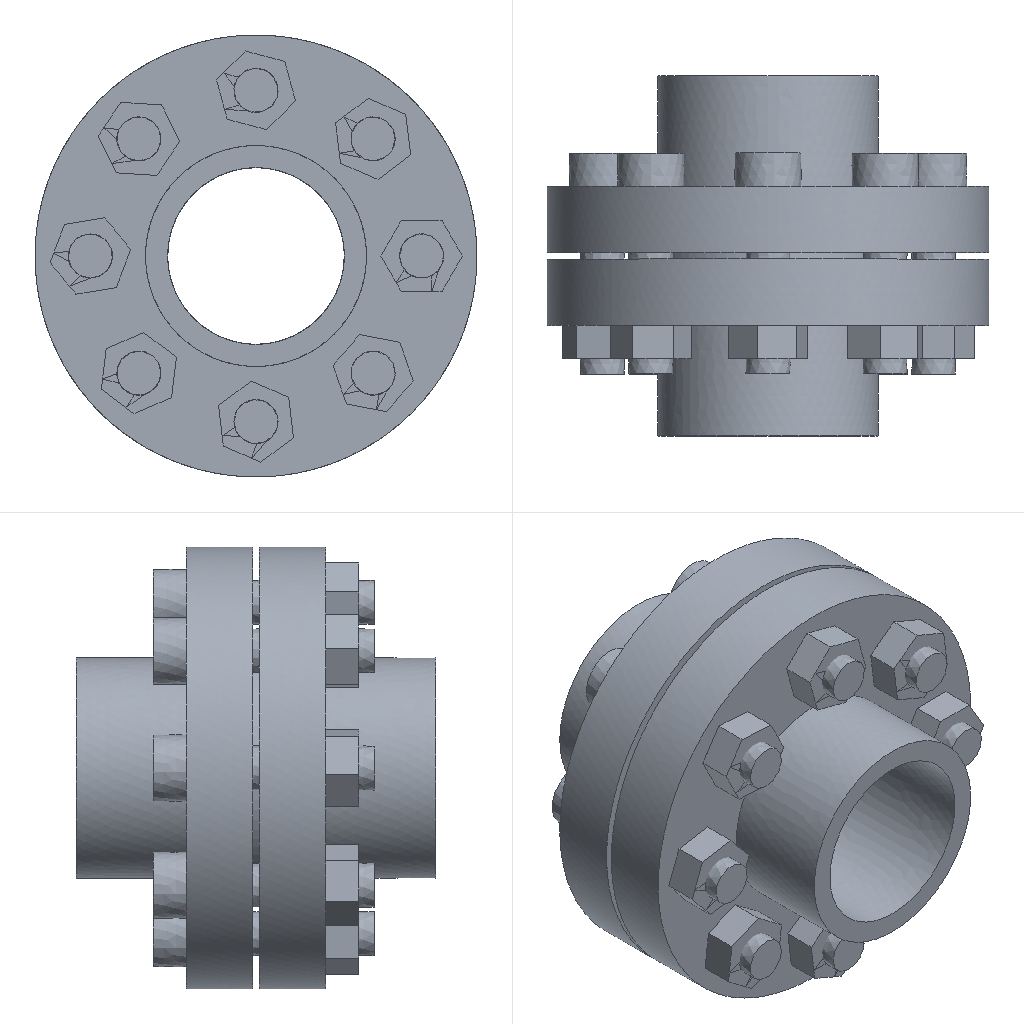Simulation study | ansys workbench
Set-up summary:
category,name,step,type,value,unit,region
solver,ansys_workbench
units,mm-N-s-tonne (MPa),,stated,"/units,MPA"
analysis,LS1,,static
load_step,LS1,LS1,static,nsubst=1; time=1
load_step,LS2,LS2,static,nsubst=1; time=2
mesh,nodes,,,148015
mesh,elements,,,97860
element_type,SOLID187,,,87205
element_type,SURF154,,,4076
element_type,TARGE170,,,2874
element_type,CONTA174,,,2874
element_type,SOLID186,,,831
material,Structural Steel,,E,200000,tonne s^-2 mm^-1
material,Structural Steel,,nu,0.3
material,Structural Steel,,density,7.85e-09,tonne mm^-3
material,Structural Steel,,conductivity,60.5,tonne mm s^-3 C^-1
material,Structural Steel,,specific_heat,4.34e+08,mm^2 s^-2 C^-1
material,Structural Steel,,cte,1.2e-05,C^-1
material,Structural Steel,,permeability,10000
material,Structural Steel,,resistivity,0.00017,ohm mm
material,Y?,,E,43,tonne s^-2 mm^-1
material,Y?,,nu,0.4995
material,Y?,,density,1.2e-09,tonne mm^-3
load,Define Pressure Using Surface Effect Elements,LS1,pressure,0.6,,SURF154 #56
load,Define Force Using Surface Effect Elements,LS1,surface-effect pres face 2,-11.318,,SURF154 #57
load,Define Force Using Surface Effect Elements,LS1,surface-effect pres face 2,-19.806,,SURF154 #58
load,Define Force Using Surface Effect Elements,LS1,surface-effect pres face 2,-19.806,,SURF154 #59
load,Define Force Using Surface Effect Elements,LS1,surface-effect pres face 2,-19.806,,SURF154 #60
load,Define Force Using Surface Effect Elements,LS1,surface-effect pres face 2,-28.295,,SURF154 #61
load,Define Force Using Surface Effect Elements,LS1,surface-effect pres face 2,-19.806,,SURF154 #62
load,Define Force Using Surface Effect Elements,LS1,surface-effect pres face 2,-19.806,,SURF154 #63
load,Define Force Using Surface Effect Elements,LS1,surface-effect pres face 2,-19.806,,SURF154 #64
bc,Fixed Supports,model,fixed,[dofs=ALL],,_FIXEDSU
contact,Contact Region,,bonded (always),element=CONTA174
contact,Contact Region 2,,bonded (always),element=CONTA174
contact,Contact Region 3,,bonded (always),element=CONTA174
contact,Contact Region 4,,bonded (always),element=CONTA174
contact,Contact Region 5,,bonded (always),element=CONTA174
contact,Contact Region 6,,bonded (always),element=CONTA174
contact,Contact Region 7,,bonded (always),element=CONTA174
contact,Contact Region 8,,bonded (always),element=CONTA174
contact,Contact Region,,bonded (always),element=CONTA174
contact,Contact Region 2,,bonded (always),element=CONTA174
contact,Contact Region 3,,bonded (always),element=CONTA174
contact,Contact Region 4,,bonded (always),element=CONTA174
contact,Contact Region 5,,bonded (always),element=CONTA174
contact,Contact Region 6,,bonded (always),element=CONTA174
contact,Contact Region 7,,bonded (always),element=CONTA174
contact,Contact Region 8,,bonded (always),element=CONTA174
contact,Frictional - falan\____-____2 ? dianpian\____-____1,,standard (frictionless/frictional),friction=0.15; element=CONTA174
contact,Frictional - falan\____-____2 ? dianpian\____-____1,,standard (frictionless/frictional),friction=0.15; element=CONTA174
named_set,_FIXEDSU,,node,3130
Ansys APDL input file, long lists of numbers shortened:
/batch
/config,noeldb,1     ! force off writing results to database
*get,_wallstrt,active,,time,wall
! ANSYS input file written by Workbench version 2021 R1
! File used for geometry attach:
/title,________--____ (C5)
*DIM,_wb_ProjectScratch_dir,string,248
_wb_ProjectScratch_dir(1) = ''
*DIM,_wb_SolverFiles_dir,string,248
_wb_SolverFiles_dir(1) = ''
*DIM,_wb_userfiles_dir,string,248
_wb_userfiles_dir(1) = ''
/com,--- Data in consistent NMM units. See Solving Units in the help system for more information.
/units,MPA
/nopr
/wb,file,start              !  signify a WB generated input file
/prep7
! Turn off shape checking because checks already performed inside WB mesher.
! See help system for more information.
SHPP,OFF,,NOWARN
/nolist
etcon,set             ! allow ANSYS to choose best KEYOP's for 180x elements, resets any applicable keyopt to MAPDL defaults
/com,*********** Nodes for the whole assembly ***********
nblock,3,,162816
(1i9,3e20.9e3)
        1     6.900000000E+01     3.000000000E+01    -8.000000000E+00
! (148014 more lines like these left out)
-1
/wb,elem,start            !  set before creation of elements
/com,*********** Elements for Body 1 "falan\____-____2" ***********
et,1,187
eblock,19,solid,,36424
(19i9)
        1        1        1        1        0        0        0        0       10        0    14541    31996    32136    35193    35172    70338    71087    70341    70340
! (72847 more lines like these left out)
-1
/com,*********** Elements for Body 2 "falan\____-____2" ***********
et,2,187
eblock,19,solid,,36424
(19i9)
        2        2        2        2        0        0        0        0       10        0    50965    90268    90408    93465    93444   128610   129359   128613   128612
! (72847 more lines like these left out)
-1
/com,*********** Elements for Body 3 "M20-LD\____-____2" ***********
et,3,187
eblock,19,solid,,1785
(19i9)
        3        3        3        3        0        0        0        0       10        0     3549     6406     6596     6715     6599     7874     8912     7876     7875
! (3569 more lines like these left out)
-1
/com,*********** Elements for Body 4 "M20-LD\____-____2" ***********
et,4,187
eblock,19,solid,,1782
(19i9)
        4        4        4        4        0        0        0        0       10        0    10977    20599    20793    20907    20796    22051    23108    22053    22052
! (3563 more lines like these left out)
-1
/com,*********** Elements for Body 5 "M20-LD\____-____2" ***********
et,5,187
eblock,19,solid,,1769
(19i9)
        5        5        5        5        0        0        0        0       10        0     1780     3524     3528     3611     3595     5949     5982     5958     5956
! (3537 more lines like these left out)
-1
! (14 more sections like these left out)
/wb,elem,end               !  done creating elements
/com,*********** Send User Defined Coordinate System(s) ***********
csys,0
toffst,273.15,  ! Temperature offset from absolute zero
/com,*********** Set Reference Temperature ***********
tref,22.
/wb,mat,start              !  starting to send materials
/com,*********** Send Materials ***********
Temperature = 'TEMP' ! Temperature
MP,DENS,1,7.85e-09,	! tonne mm^-3
MP,ALPX,1,1.2e-05,	! C^-1
MP,C,1,434000000,	! mm^2 s^-2 C^-1
MP,KXX,1,60.5,	! tonne mm s^-3 C^-1
MP,RSVX,1,0.00017,	! ohm mm
MP,EX,1,200000,	! tonne s^-2 mm^-1
MP,NUXY,1,0.3,
MP,MURX,1,10000,
Temperature = 'TEMP' ! Temperature
MP,DENS,2,7.85e-09,	! tonne mm^-3
MP,ALPX,2,1.2e-05,	! C^-1
MP,C,2,434000000,	! mm^2 s^-2 C^-1
MP,KXX,2,60.5,	! tonne mm s^-3 C^-1
MP,RSVX,2,0.00017,	! ohm mm
MP,EX,2,200000,	! tonne s^-2 mm^-1
MP,NUXY,2,0.3,
MP,MURX,2,10000,
Temperature = 'TEMP' ! Temperature
MP,DENS,3,7.85e-09,	! tonne mm^-3
MP,ALPX,3,1.2e-05,	! C^-1
MP,C,3,434000000,	! mm^2 s^-2 C^-1
MP,KXX,3,60.5,	! tonne mm s^-3 C^-1
MP,RSVX,3,0.00017,	! ohm mm
MP,EX,3,200000,	! tonne s^-2 mm^-1
MP,NUXY,3,0.3,
MP,MURX,3,10000,
Temperature = 'TEMP' ! Temperature
MP,DENS,4,7.85e-09,	! tonne mm^-3
MP,ALPX,4,1.2e-05,	! C^-1
MP,C,4,434000000,	! mm^2 s^-2 C^-1
MP,KXX,4,60.5,	! tonne mm s^-3 C^-1
MP,RSVX,4,0.00017,	! ohm mm
MP,EX,4,200000,	! tonne s^-2 mm^-1
MP,NUXY,4,0.3,
MP,MURX,4,10000,
Temperature = 'TEMP' ! Temperature
MP,DENS,5,7.85e-09,	! tonne mm^-3
MP,ALPX,5,1.2e-05,	! C^-1
MP,C,5,434000000,	! mm^2 s^-2 C^-1
MP,KXX,5,60.5,	! tonne mm s^-3 C^-1
MP,RSVX,5,0.00017,	! ohm mm
MP,EX,5,200000,	! tonne s^-2 mm^-1
MP,NUXY,5,0.3,
MP,MURX,5,10000,
Temperature = 'TEMP' ! Temperature
MP,DENS,6,7.85e-09,	! tonne mm^-3
MP,ALPX,6,1.2e-05,	! C^-1
MP,C,6,434000000,	! mm^2 s^-2 C^-1
MP,KXX,6,60.5,	! tonne mm s^-3 C^-1
MP,RSVX,6,0.00017,	! ohm mm
MP,EX,6,200000,	! tonne s^-2 mm^-1
MP,NUXY,6,0.3,
MP,MURX,6,10000,
Temperature = 'TEMP' ! Temperature
MP,DENS,7,7.85e-09,	! tonne mm^-3
MP,ALPX,7,1.2e-05,	! C^-1
MP,C,7,434000000,	! mm^2 s^-2 C^-1
MP,KXX,7,60.5,	! tonne mm s^-3 C^-1
MP,RSVX,7,0.00017,	! ohm mm
MP,EX,7,200000,	! tonne s^-2 mm^-1
MP,NUXY,7,0.3,
MP,MURX,7,10000,
Temperature = 'TEMP' ! Temperature
MP,DENS,8,7.85e-09,	! tonne mm^-3
MP,ALPX,8,1.2e-05,	! C^-1
MP,C,8,434000000,	! mm^2 s^-2 C^-1
MP,KXX,8,60.5,	! tonne mm s^-3 C^-1
MP,RSVX,8,0.00017,	! ohm mm
MP,EX,8,200000,	! tonne s^-2 mm^-1
MP,NUXY,8,0.3,
MP,MURX,8,10000,
Temperature = 'TEMP' ! Temperature
MP,DENS,9,7.85e-09,	! tonne mm^-3
MP,ALPX,9,1.2e-05,	! C^-1
MP,C,9,434000000,	! mm^2 s^-2 C^-1
MP,KXX,9,60.5,	! tonne mm s^-3 C^-1
MP,RSVX,9,0.00017,	! ohm mm
MP,EX,9,200000,	! tonne s^-2 mm^-1
! (86 more lines like these left out)
/wb,mat,end                !  done sending materials
!************************* Model Summary ********************
!falan\____-____2,	结构钢,	matid,	1
!falan\____-____2,	结构钢,	matid,	2
!M20-LD\____-____2,	结构钢,	matid,	3
!M20-LD\____-____2,	结构钢,	matid,	4
!M20-LD\____-____2,	结构钢,	matid,	5
!M20-LD\____-____2,	结构钢,	matid,	6
!M20-LD\____-____2,	结构钢,	matid,	7
!M20-LD\____-____2,	结构钢,	matid,	8
!M20-LD\____-____2,	结构钢,	matid,	9
!M20-LD\____-____2,	结构钢,	matid,	10
!dianpian\____-____1,	Y形圈,	matid,	11
!M20-LM\____-____1,	结构钢,	matid,	12
!M20-LM\____-____1,	结构钢,	matid,	13
!M20-LM\____-____1,	结构钢,	matid,	14
!M20-LM\____-____1,	结构钢,	matid,	15
!M20-LM\____-____1,	结构钢,	matid,	16
!M20-LM\____-____1,	结构钢,	matid,	17
!M20-LM\____-____1,	结构钢,	matid,	18
!M20-LM\____-____1,	结构钢,	matid,	19
!************************* End Model Summary ********************
! get the diagonal of the bounding box. Needed later for other things
*get,_xmin,node,,mnloc,x
*get,_ymin,node,,mnloc,y
*get,_zmin,node,,mnloc,z
*get,_xmax,node,,mxloc,x
*get,_ymax,node,,mxloc,y
*get,_zmax,node,,mxloc,z
_ASMDIAG=(_xmax-_xmin)*(_xmax-_xmin)+(_ymax-_ymin)*(_ymax-_ymin)+(_zmax-_zmin)*(_zmax-_zmin)
_ASMDIAG=SQRT(_ASMDIAG)
/wb,contact,start          !  starting to send contact
/com,*********** Create Contact "接触区域" ***********
/com,            Real Constant Set For Above Contact Is 21 & 20
*set,tid,21
*set,cid,20
r,tid
r,cid
et,tid,170
et,cid,174
eblock,10,,,52
(15i9)
   114315       21       21       21        0    26792    27303    28168    28168    36267    39875    28168    36268
! (51 more lines like these left out)
-1
eblock,10,,,52
(15i9)
   114367       20       20       20        0    26792    27303    28168    28168    36267    39875    28168    36268
! (51 more lines like these left out)
-1
eblock,10,,,33
(15i9)
   114419       20       21       20        0     6217     6278     6257     6257     6720     7023     6257     6718
! (32 more lines like these left out)
-1
eblock,10,,,33
(15i9)
   114452       21       20       21        0     6217     6278     6257     6257     6720     7023     6257     6718
! (32 more lines like these left out)
-1
keyo,cid,8,2               ! auto create asymmetric contact (from Program Controlled setting)
keyo,cid,10,0              ! adjust contact stiffness each NR iteration (from Program Controlled setting)
keyo,cid,12,5              ! bonded always
keyo,cid,18,1              ! small sliding turned on by application
keyo,cid,2,0               ! augmented Lagrange (from Program Controlled setting)
keyo,cid,4,0               ! on Gauss point (from Program Controlled setting)
keyo,cid,9,1               ! ignore initial gaps/penetration
keyo,cid,7,0               ! No Prediction
rmod,tid,3,1.       ! FKN
rmod,tid,5,0.       ! ICONT
rmod,tid,6,0.       ! PINB
rmod,tid,10,0.      ! CNOF
rmod,tid,12,0.      ! FKT
rmod,tid,36,1254    ! WB DSID
rmod,cid,3,1.       ! FKN
rmod,cid,5,0.       ! ICONT
rmod,cid,6,0.       ! PINB
rmod,cid,10,0.      ! CNOF
rmod,cid,12,0.      ! FKT
rmod,cid,36,1254    ! WB DSID
/com,*********** Create Contact "接触区域 2" ***********
/com,            Real Constant Set For Above Contact Is 23 & 22
*set,tid,23
*set,cid,22
r,tid
r,cid
et,tid,170
et,cid,174
eblock,10,,,50
(15i9)
   114485       23       23       23        0    28204    28345    28409    28409    46108    47141    28409    46109
! (49 more lines like these left out)
-1
eblock,10,,,50
(15i9)
   114535       22       22       22        0    28204    28345    28409    28409    46108    47141    28409    46109
! (49 more lines like these left out)
-1
eblock,10,,,33
(15i9)
   114585       22       23       22        0    20410    20471    20450    20450    20913    21213    20450    20910
! (32 more lines like these left out)
-1
eblock,10,,,33
(15i9)
   114618       23       22       23        0    20410    20471    20450    20450    20913    21213    20450    20910
! (32 more lines like these left out)
-1
keyo,cid,8,2               ! auto create asymmetric contact (from Program Controlled setting)
keyo,cid,10,0              ! adjust contact stiffness each NR iteration (from Program Controlled setting)
keyo,cid,12,5              ! bonded always
keyo,cid,18,1              ! small sliding turned on by application
keyo,cid,2,0               ! augmented Lagrange (from Program Controlled setting)
keyo,cid,4,0               ! on Gauss point (from Program Controlled setting)
keyo,cid,9,1               ! ignore initial gaps/penetration
keyo,cid,7,0               ! No Prediction
rmod,tid,3,1.       ! FKN
rmod,tid,5,0.       ! ICONT
rmod,tid,6,0.       ! PINB
rmod,tid,10,0.      ! CNOF
rmod,tid,12,0.      ! FKT
rmod,tid,36,1257    ! WB DSID
rmod,cid,3,1.       ! FKN
rmod,cid,5,0.       ! ICONT
rmod,cid,6,0.       ! PINB
rmod,cid,10,0.      ! CNOF
rmod,cid,12,0.      ! FKT
rmod,cid,36,1257    ! WB DSID
/com,*********** Create Contact "接触区域 3" ***********
/com,            Real Constant Set For Above Contact Is 25 & 24
*set,tid,25
*set,cid,24
r,tid
r,cid
et,tid,170
et,cid,174
eblock,10,,,47
(15i9)
   114651       25       25       25        0    28197    28481    28599    28599    46040    47853    28599    46042
! (46 more lines like these left out)
-1
eblock,10,,,47
(15i9)
   114698       24       24       24        0    28197    28481    28599    28599    46040    47853    28599    46042
! (46 more lines like these left out)
-1
eblock,10,,,33
(15i9)
   114745       24       25       24        0     3116     3177     3156     3156     3616     3907     3156     3614
! (32 more lines like these left out)
-1
eblock,10,,,33
(15i9)
   114778       25       24       25        0     3116     3177     3156     3156     3616     3907     3156     3614
! (32 more lines like these left out)
-1
keyo,cid,8,2               ! auto create asymmetric contact (from Program Controlled setting)
keyo,cid,10,0              ! adjust contact stiffness each NR iteration (from Program Controlled setting)
keyo,cid,12,5              ! bonded always
keyo,cid,18,1              ! small sliding turned on by application
keyo,cid,2,0               ! augmented Lagrange (from Program Controlled setting)
keyo,cid,4,0               ! on Gauss point (from Program Controlled setting)
keyo,cid,9,1               ! ignore initial gaps/penetration
keyo,cid,7,0               ! No Prediction
rmod,tid,3,1.       ! FKN
rmod,tid,5,0.       ! ICONT
rmod,tid,6,0.       ! PINB
rmod,tid,10,0.      ! CNOF
rmod,tid,12,0.      ! FKT
rmod,tid,36,1260    ! WB DSID
rmod,cid,3,1.       ! FKN
rmod,cid,5,0.       ! ICONT
rmod,cid,6,0.       ! PINB
rmod,cid,10,0.      ! CNOF
rmod,cid,12,0.      ! FKT
rmod,cid,36,1260    ! WB DSID
/com,*********** Create Contact "接触区域 4" ***********
/com,            Real Constant Set For Above Contact Is 27 & 26
*set,tid,27
*set,cid,26
r,tid
r,cid
et,tid,170
et,cid,174
eblock,10,,,62
(15i9)
   114811       27       27       27        0    28129    28528    28315    28315    45441    46948    28315    45439
! (61 more lines like these left out)
-1
eblock,10,,,62
(15i9)
   114873       26       26       26        0    28129    28528    28315    28315    45441    46948    28315    45439
! (61 more lines like these left out)
-1
eblock,10,,,33
(15i9)
   114935       26       27       26        0        1       62       41       41      503      803       41      501
! (32 more lines like these left out)
-1
eblock,10,,,33
(15i9)
   114968       27       26       27        0        1       62       41       41      503      803       41      501
! (32 more lines like these left out)
-1
keyo,cid,8,2               ! auto create asymmetric contact (from Program Controlled setting)
keyo,cid,10,0              ! adjust contact stiffness each NR iteration (from Program Controlled setting)
keyo,cid,12,5              ! bonded always
keyo,cid,18,1              ! small sliding turned on by application
keyo,cid,2,0               ! augmented Lagrange (from Program Controlled setting)
keyo,cid,4,0               ! on Gauss point (from Program Controlled setting)
keyo,cid,9,1               ! ignore initial gaps/penetration
keyo,cid,7,0               ! No Prediction
rmod,tid,3,1.       ! FKN
rmod,tid,5,0.       ! ICONT
rmod,tid,6,0.       ! PINB
rmod,tid,10,0.      ! CNOF
rmod,tid,12,0.      ! FKT
rmod,tid,36,1263    ! WB DSID
rmod,cid,3,1.       ! FKN
rmod,cid,5,0.       ! ICONT
rmod,cid,6,0.       ! PINB
rmod,cid,10,0.      ! CNOF
rmod,cid,12,0.      ! FKT
rmod,cid,36,1263    ! WB DSID
/com,*********** Create Contact "接触区域 5" ***********
/com,            Real Constant Set For Above Contact Is 29 & 28
*set,tid,29
*set,cid,28
r,tid
r,cid
et,tid,170
et,cid,174
eblock,10,,,55
(15i9)
   115001       29       29       29        0    28159    28355    28354    28354    45708    47194    28354    45707
! (54 more lines like these left out)
-1
eblock,10,,,55
(15i9)
   115056       28       28       28        0    28159    28355    28354    28354    45708    47194    28354    45707
! (54 more lines like these left out)
-1
eblock,10,,,33
(15i9)
   115111       28       29       28        0    12487    12548    12527    12527    12993    13291    12527    12991
! (32 more lines like these left out)
-1
eblock,10,,,33
(15i9)
   115144       29       28       29        0    12487    12548    12527    12527    12993    13291    12527    12991
! (32 more lines like these left out)
-1
keyo,cid,8,2               ! auto create asymmetric contact (from Program Controlled setting)
keyo,cid,10,0              ! adjust contact stiffness each NR iteration (from Program Controlled setting)
keyo,cid,12,5              ! bonded always
keyo,cid,18,1              ! small sliding turned on by application
keyo,cid,2,0               ! augmented Lagrange (from Program Controlled setting)
keyo,cid,4,0               ! on Gauss point (from Program Controlled setting)
keyo,cid,9,1               ! ignore initial gaps/penetration
keyo,cid,7,0               ! No Prediction
rmod,tid,3,1.       ! FKN
rmod,tid,5,0.       ! ICONT
rmod,tid,6,0.       ! PINB
rmod,tid,10,0.      ! CNOF
rmod,tid,12,0.      ! FKT
rmod,tid,36,1266    ! WB DSID
rmod,cid,3,1.       ! FKN
rmod,cid,5,0.       ! ICONT
rmod,cid,6,0.       ! PINB
rmod,cid,10,0.      ! CNOF
rmod,cid,12,0.      ! FKT
rmod,cid,36,1266    ! WB DSID
! (13 more sections like these left out)
/wb,contact,end            !  done creating contacts
/golist
/wb,load,start             !  starting to send loads
/com,*********** Fixed Supports ***********
CMBLOCK,_FIXEDSU,NODE,     3130
(8i10)
     85012     85018     85019     85020     85021     85022     85023     85024
! (391 more lines like these left out)
cmsel,s,_FIXEDSU
d,all,all
nsel,all
/com,*********** Define Pressure Using Surface Effect Elements ***********
et,56,154
eblock,10,,,3692
(15i9)
   120063       56       56       56        0    26680    28692    28693    28693    35411    48843    28693    35412
! (3691 more lines like these left out)
-1
esel,s,type,,56
keyop,56,7,0                ! Use deformed area for application of load
esel,all
*DIM,_loadvari835,TABLE,3,1,1,TIME,
! Time values
_loadvari835(1,0,1) = 0.
_loadvari835(2,0,1) = 1.
_loadvari835(3,0,1) = 2.
! Load values
_loadvari835(1,1,1) = 0.
_loadvari835(2,1,1) = 0.
_loadvari835(3,1,1) = 0.6
/com,*********** Define Force Using Surface Effect Elements ***********
local,12,0,0.,0.,0.,0.,0.,0.
csys,0
et,57,154
eblock,10,,,48
(15i9)
   123755       57       57       57       12      329      332      341      341     2375     2403      341     2379
! (47 more lines like these left out)
-1
esel,s,type,,57
keyop,57,2,1                ! Apply load in local coordinate system
keyop,57,7,1                ! Use original area so load is constant in large deformation
esel,all
*DIM,_loadvari871x,TABLE,3,1,1,TIME,
! Time values
_loadvari871x(1,0,1) = 0.
_loadvari871x(2,0,1) = 1.
_loadvari871x(3,0,1) = 2.
! Load values
_loadvari871x(1,1,1) = 0.
_loadvari871x(2,1,1) = 0.
_loadvari871x(3,1,1) = 0.
*DIM,_loadvari871y,TABLE,3,1,1,TIME,
! Time values
_loadvari871y(1,0,1) = 0.
_loadvari871y(2,0,1) = 1.
_loadvari871y(3,0,1) = 2.
! Load values
_loadvari871y(1,1,1) = 0.
_loadvari871y(2,1,1) = -11.318
_loadvari871y(3,1,1) = -11.318
*DIM,_loadvari871z,TABLE,3,1,1,TIME,
! Time values
_loadvari871z(1,0,1) = 0.
_loadvari871z(2,0,1) = 1.
_loadvari871z(3,0,1) = 2.
! Load values
_loadvari871z(1,1,1) = 0.
_loadvari871z(2,1,1) = 0.
_loadvari871z(3,1,1) = 0.
/com,*********** Define Force Using Surface Effect Elements ***********
local,13,0,0.,0.,0.,0.,0.,0.
csys,0
et,58,154
eblock,10,,,48
(15i9)
   123803       58       58       58       13    12815    12818    12827    12827    14879    14908    12827    14883
! (47 more lines like these left out)
-1
esel,s,type,,58
keyop,58,2,1                ! Apply load in local coordinate system
keyop,58,7,1                ! Use original area so load is constant in large deformation
esel,all
*DIM,_loadvari879x,TABLE,3,1,1,TIME,
! Time values
_loadvari879x(1,0,1) = 0.
_loadvari879x(2,0,1) = 1.
_loadvari879x(3,0,1) = 2.
! Load values
_loadvari879x(1,1,1) = 0.
_loadvari879x(2,1,1) = 0.
_loadvari879x(3,1,1) = 0.
*DIM,_loadvari879y,TABLE,3,1,1,TIME,
! Time values
_loadvari879y(1,0,1) = 0.
_loadvari879y(2,0,1) = 1.
_loadvari879y(3,0,1) = 2.
! Load values
_loadvari879y(1,1,1) = 0.
_loadvari879y(2,1,1) = -19.806
_loadvari879y(3,1,1) = -19.806
*DIM,_loadvari879z,TABLE,3,1,1,TIME,
! Time values
_loadvari879z(1,0,1) = 0.
_loadvari879z(2,0,1) = 1.
_loadvari879z(3,0,1) = 2.
! Load values
_loadvari879z(1,1,1) = 0.
_loadvari879z(2,1,1) = 0.
_loadvari879z(3,1,1) = 0.
/com,*********** Define Force Using Surface Effect Elements ***********
local,14,0,0.,0.,0.,0.,0.,0.
csys,0
et,59,154
eblock,10,,,48
(15i9)
   123851       59       59       59       14     9668     9671     9680     9680    11729    11755     9680    11733
! (47 more lines like these left out)
-1
esel,s,type,,59
keyop,59,2,1                ! Apply load in local coordinate system
keyop,59,7,1                ! Use original area so load is constant in large deformation
esel,all
*DIM,_loadvari881x,TABLE,3,1,1,TIME,
! Time values
_loadvari881x(1,0,1) = 0.
_loadvari881x(2,0,1) = 1.
_loadvari881x(3,0,1) = 2.
! Load values
_loadvari881x(1,1,1) = 0.
_loadvari881x(2,1,1) = 0.
_loadvari881x(3,1,1) = 0.
*DIM,_loadvari881y,TABLE,3,1,1,TIME,
! Time values
_loadvari881y(1,0,1) = 0.
_loadvari881y(2,0,1) = 1.
_loadvari881y(3,0,1) = 2.
! Load values
_loadvari881y(1,1,1) = 0.
_loadvari881y(2,1,1) = -19.806
_loadvari881y(3,1,1) = -19.806
*DIM,_loadvari881z,TABLE,3,1,1,TIME,
! Time values
_loadvari881z(1,0,1) = 0.
_loadvari881z(2,0,1) = 1.
_loadvari881z(3,0,1) = 2.
! Load values
_loadvari881z(1,1,1) = 0.
_loadvari881z(2,1,1) = 0.
_loadvari881z(3,1,1) = 0.
/com,*********** Define Force Using Surface Effect Elements ***********
local,15,0,0.,0.,0.,0.,0.,0.
csys,0
et,60,154
eblock,10,,,48
(15i9)
   123899       60       60       60       15    15974    15977    15986    15986    18062    18089    15986    18066
! (47 more lines like these left out)
-1
esel,s,type,,60
keyop,60,2,1                ! Apply load in local coordinate system
keyop,60,7,1                ! Use original area so load is constant in large deformation
esel,all
*DIM,_loadvari883x,TABLE,3,1,1,TIME,
! Time values
_loadvari883x(1,0,1) = 0.
_loadvari883x(2,0,1) = 1.
_loadvari883x(3,0,1) = 2.
! Load values
_loadvari883x(1,1,1) = 0.
_loadvari883x(2,1,1) = 0.
_loadvari883x(3,1,1) = 0.
*DIM,_loadvari883y,TABLE,3,1,1,TIME,
! Time values
_loadvari883y(1,0,1) = 0.
_loadvari883y(2,0,1) = 1.
_loadvari883y(3,0,1) = 2.
! Load values
_loadvari883y(1,1,1) = 0.
_loadvari883y(2,1,1) = -19.806
_loadvari883y(3,1,1) = -19.806
*DIM,_loadvari883z,TABLE,3,1,1,TIME,
! Time values
_loadvari883z(1,0,1) = 0.
_loadvari883z(2,0,1) = 1.
_loadvari883z(3,0,1) = 2.
! Load values
_loadvari883z(1,1,1) = 0.
_loadvari883z(2,1,1) = 0.
_loadvari883z(3,1,1) = 0.
/com,*********** Define Force Using Surface Effect Elements ***********
local,16,0,0.,0.,0.,0.,0.,0.
csys,0
et,61,154
eblock,10,,,48
(15i9)
   123947       61       61       61       16    23856    23859    23868    23868    25905    25932    23868    25909
! (47 more lines like these left out)
-1
esel,s,type,,61
keyop,61,2,1                ! Apply load in local coordinate system
keyop,61,7,1                ! Use original area so load is constant in large deformation
esel,all
*DIM,_loadvari885x,TABLE,3,1,1,TIME,
! Time values
_loadvari885x(1,0,1) = 0.
_loadvari885x(2,0,1) = 1.
_loadvari885x(3,0,1) = 2.
! Load values
_loadvari885x(1,1,1) = 0.
_loadvari885x(2,1,1) = 0.
_loadvari885x(3,1,1) = 0.
*DIM,_loadvari885y,TABLE,3,1,1,TIME,
! Time values
_loadvari885y(1,0,1) = 0.
_loadvari885y(2,0,1) = 1.
_loadvari885y(3,0,1) = 2.
! Load values
_loadvari885y(1,1,1) = 0.
_loadvari885y(2,1,1) = -28.295
_loadvari885y(3,1,1) = -28.295
*DIM,_loadvari885z,TABLE,3,1,1,TIME,
! Time values
_loadvari885z(1,0,1) = 0.
_loadvari885z(2,0,1) = 1.
_loadvari885z(3,0,1) = 2.
! Load values
_loadvari885z(1,1,1) = 0.
_loadvari885z(2,1,1) = 0.
_loadvari885z(3,1,1) = 0.
/com,*********** Define Force Using Surface Effect Elements ***********
local,17,0,0.,0.,0.,0.,0.,0.
csys,0
et,62,154
eblock,10,,,48
(15i9)
   123995       62       62       62       17     6545     6548     6557     6557     8602     8627     6557     8606
! (47 more lines like these left out)
-1
esel,s,type,,62
keyop,62,2,1                ! Apply load in local coordinate system
keyop,62,7,1                ! Use original area so load is constant in large deformation
esel,all
*DIM,_loadvari887x,TABLE,3,1,1,TIME,
! Time values
_loadvari887x(1,0,1) = 0.
_loadvari887x(2,0,1) = 1.
_loadvari887x(3,0,1) = 2.
! Load values
_loadvari887x(1,1,1) = 0.
_loadvari887x(2,1,1) = 0.
_loadvari887x(3,1,1) = 0.
*DIM,_loadvari887y,TABLE,3,1,1,TIME,
! Time values
_loadvari887y(1,0,1) = 0.
_loadvari887y(2,0,1) = 1.
_loadvari887y(3,0,1) = 2.
! Load values
_loadvari887y(1,1,1) = 0.
_loadvari887y(2,1,1) = -19.806
_loadvari887y(3,1,1) = -19.806
*DIM,_loadvari887z,TABLE,3,1,1,TIME,
! Time values
_loadvari887z(1,0,1) = 0.
_loadvari887z(2,0,1) = 1.
_loadvari887z(3,0,1) = 2.
! Load values
_loadvari887z(1,1,1) = 0.
_loadvari887z(2,1,1) = 0.
_loadvari887z(3,1,1) = 0.
/com,*********** Define Force Using Surface Effect Elements ***********
local,18,0,0.,0.,0.,0.,0.,0.
csys,0
et,63,154
eblock,10,,,48
(15i9)
   124043       63       63       63       18    20738    20741    20750    20750    22782    22809    20750    22786
! (47 more lines like these left out)
-1
esel,s,type,,63
keyop,63,2,1                ! Apply load in local coordinate system
keyop,63,7,1                ! Use original area so load is constant in large deformation
esel,all
*DIM,_loadvari889x,TABLE,3,1,1,TIME,
! Time values
_loadvari889x(1,0,1) = 0.
_loadvari889x(2,0,1) = 1.
_loadvari889x(3,0,1) = 2.
! Load values
_loadvari889x(1,1,1) = 0.
_loadvari889x(2,1,1) = 0.
_loadvari889x(3,1,1) = 0.
*DIM,_loadvari889y,TABLE,3,1,1,TIME,
! Time values
_loadvari889y(1,0,1) = 0.
_loadvari889y(2,0,1) = 1.
_loadvari889y(3,0,1) = 2.
! Load values
_loadvari889y(1,1,1) = 0.
_loadvari889y(2,1,1) = -19.806
_loadvari889y(3,1,1) = -19.806
*DIM,_loadvari889z,TABLE,3,1,1,TIME,
! Time values
_loadvari889z(1,0,1) = 0.
_loadvari889z(2,0,1) = 1.
_loadvari889z(3,0,1) = 2.
! Load values
_loadvari889z(1,1,1) = 0.
_loadvari889z(2,1,1) = 0.
_loadvari889z(3,1,1) = 0.
/com,*********** Define Force Using Surface Effect Elements ***********
local,19,0,0.,0.,0.,0.,0.,0.
csys,0
et,64,154
eblock,10,,,48
(15i9)
   124091       64       64       64       19     3444     3447     3456     3456     5489     5515     3456     5493
! (47 more lines like these left out)
-1
esel,s,type,,64
keyop,64,2,1                ! Apply load in local coordinate system
keyop,64,7,1                ! Use original area so load is constant in large deformation
esel,all
*DIM,_loadvari891x,TABLE,3,1,1,TIME,
! Time values
_loadvari891x(1,0,1) = 0.
_loadvari891x(2,0,1) = 1.
_loadvari891x(3,0,1) = 2.
! Load values
_loadvari891x(1,1,1) = 0.
_loadvari891x(2,1,1) = 0.
_loadvari891x(3,1,1) = 0.
*DIM,_loadvari891y,TABLE,3,1,1,TIME,
! Time values
_loadvari891y(1,0,1) = 0.
_loadvari891y(2,0,1) = 1.
_loadvari891y(3,0,1) = 2.
! Load values
_loadvari891y(1,1,1) = 0.
_loadvari891y(2,1,1) = -19.806
_loadvari891y(3,1,1) = -19.806
*DIM,_loadvari891z,TABLE,3,1,1,TIME,
! Time values
_loadvari891z(1,0,1) = 0.
_loadvari891z(2,0,1) = 1.
_loadvari891z(3,0,1) = 2.
! Load values
_loadvari891z(1,1,1) = 0.
_loadvari891z(2,1,1) = 0.
_loadvari891z(3,1,1) = 0.
esel,all
/gst,on,on
fini
*get,_numnode,node,0,count
*get,_numelem,elem,0,count
*get, _MAXELEMNUM, elem, 0, NUM, MAX
*get, _MAXNODENUM, node, 0, NUM, MAX
*get, _MAXELEMTYPE, etyp, 0, NUM, MAX
*get, _MAXREALCONST, real, 0, NUM, MAX
/go
/wb,load,end               !  done creating loads
/com,--- Number of total nodes = %_numnode%
/com,--- Number of contact elements = 9824
/com,--- Number of spring elements = 0
/com,--- Number of bearing elements = 0
/com,--- Number of solid elements = 88036
/com,--- Number of condensed parts = 0
/com,--- Number of total elements = %_numelem%
*get,_wallbsol,active,,time,wall
/com,****************************************************************************
/com,*************************    SOLUTION       ********************************
/com,****************************************************************************
/solu
antype,0                   ! static analysis
_thickRatio=0.526   ! Ratio of thick parts in the model
eqsl,pcg,1e-8,,,,,,1
cntr,print,1               ! print out contact info and also make no initial contact an error
dmpoption,emat,no             ! Don't combine emat file for DANSYS
dmpoption,esav,no             ! Don't combine esav file for DANSYS
nldiag,cont,iter           ! print out contact info each equilibrium iteration
rescontrol,define,last,last,,dele	   ! Program Controlled
/com,****************************************************
/com,******************* SOLVE FOR LS 1 OF 2 ****************
esel,s,type,,56
nsle
sf,all,pres,%_loadvari835%
nsel,all
esel,all
esel,s,type,,57
nsle
sfe,all,1,pres,1,%_loadvari871x%
sfe,all,2,pres,1,%_loadvari871y%
sfe,all,3,pres,1,%_loadvari871z%
esel,s,type,,58
nsle
sfe,all,1,pres,1,%_loadvari879x%
sfe,all,2,pres,1,%_loadvari879y%
sfe,all,3,pres,1,%_loadvari879z%
esel,s,type,,59
nsle
sfe,all,1,pres,1,%_loadvari881x%
sfe,all,2,pres,1,%_loadvari881y%
sfe,all,3,pres,1,%_loadvari881z%
esel,s,type,,60
nsle
sfe,all,1,pres,1,%_loadvari883x%
sfe,all,2,pres,1,%_loadvari883y%
sfe,all,3,pres,1,%_loadvari883z%
esel,s,type,,61
nsle
sfe,all,1,pres,1,%_loadvari885x%
sfe,all,2,pres,1,%_loadvari885y%
sfe,all,3,pres,1,%_loadvari885z%
esel,s,type,,62
nsle
sfe,all,1,pres,1,%_loadvari887x%
sfe,all,2,pres,1,%_loadvari887y%
sfe,all,3,pres,1,%_loadvari887z%
esel,s,type,,63
nsle
sfe,all,1,pres,1,%_loadvari889x%
sfe,all,2,pres,1,%_loadvari889y%
sfe,all,3,pres,1,%_loadvari889z%
esel,s,type,,64
nsle
sfe,all,1,pres,1,%_loadvari891x%
sfe,all,2,pres,1,%_loadvari891y%
sfe,all,3,pres,1,%_loadvari891z%
nsel,all
esel,all
esel,all
/nopr
/gopr
/nolist
autots,on                  ! Workbench Program Controlled automatic time stepping
nsub,1,10,1                ! due to presence of general nonlinear
time,1.
outres,erase
outres,all,none
outres,nsol,all,
outres,rsol,all
outres,eangl,all
outres,etmp,all
outres,veng,all
outres,strs,all,
outres,epel,all,
outres,eppl,all,
outres,cont,all,
! *********** WB SOLVE COMMAND ***********
! check interactive state
*get,ANSINTER_,active,,int
*if,ANSINTER_,ne,0,then
/eof
*endif
solve
/com *************** Write FE CONNECTORS *********
CEWRITE,file,ce,,INTE
/com,****************************************************
/com,*************** FINISHED SOLVE FOR LS 1 *************
/com,****************************************************
/com,******************* SOLVE FOR LS 2 OF 2 ****************
esel,all
/nopr
/gopr
/nolist
autots,on                  ! Workbench Program Controlled automatic time stepping
nsub,1,10,1                ! due to presence of general nonlinear
time,2.
outres,erase
outres,all,none
outres,nsol,all,
outres,rsol,all
outres,eangl,all
outres,etmp,all
outres,veng,all
outres,strs,all,
outres,epel,all,
outres,eppl,all,
outres,cont,all,
solve
/com,****************************************************
/com,*************** FINISHED SOLVE FOR LS 2 *************
*get,_wallasol,active,,time,wall
/nopr
*get,_numnode,node,0,count
*get,_numelem,elem,0,count
*get, _MAXELEMNUM, elem, 0, NUM, MAX
*get, _MAXNODENUM, node, 0, NUM, MAX,,,INTERNAL
*get, _MAXELEMTYPE, etyp, 0, NUM, MAX
*get, _MAXREALCONST, real, 0, NUM, MAX
/gopr
*get,_PCGITER,active,,solu,cgiter
/post1
xmlo,ENCODING,ISO-8859-1
xmlo,parm
/xml,parm,xml
fini
/gopr
*get,_walldone,active,,time,wall
_preptime=(_wallbsol-_wallstrt)*3600
_solvtime=(_wallasol-_wallbsol)*3600
_posttime=(_walldone-_wallasol)*3600
_totaltim=(_walldone-_wallstrt)*3600
*get,_dlbratio,active,0,solu,dlbr
*get,_combtime,active,0,solu,comb
/com,--- Total number of nodes = %_numnode%
/com,--- Total number of elements = %_numelem%
/com,--- Element load balance ratio = %_dlbratio%
/com,--- Time to combine distributed files = %_combtime%
/wb,file,end               ! done with WB generated input
Results summary:
result,analyses[0].index,,,1
result,analyses[0].system,,,SYS-2
result,analyses[0].deck,,,deck.dat
result,analyses[0].solve_status,,,completed
result,analyses[0].analysis_type,,,static
result,analyses[0].physics,,,mechanical
result,analyses[0].unit_system,,,"NMM: mm, ton, N, s, mV, mA, degC"
result,analyses[0].n_sets,,,2
result,analyses[0].load_steps[0].set,set=1,,1
result,analyses[0].load_steps[0].time_or_freq,set=1,,1
result,analyses[0].load_steps[0].max_displacement_magnitude,set=1,,3.604
result,analyses[0].load_steps[0].max_von_mises_nodal,set=1,,116.792
result,analyses[0].load_steps[0].reaction_force_sum_xyz[1],set=1,,9.72316e-10
result,analyses[0].load_steps[0].reaction_force_sum_xyz[2],set=1,,112000
result,analyses[0].load_steps[0].reaction_force_sum_xyz[3],set=1,,-8.26042e-10
result,analyses[0].load_steps[1].set,set=2,,2
result,analyses[0].load_steps[1].time_or_freq,set=2,,2
result,analyses[0].load_steps[1].max_displacement_magnitude,set=2,,3.604
result,analyses[0].load_steps[1].max_von_mises_nodal,set=2,,117.316
result,analyses[0].load_steps[1].reaction_force_sum_xyz[1],set=2,,2.38395e-08
result,analyses[0].load_steps[1].reaction_force_sum_xyz[2],set=2,,112000
result,analyses[0].load_steps[1].reaction_force_sum_xyz[3],set=2,,-1.97051e-08
result,geometry_export[0][0],,,.step
result,geometry_export[0][1],,,ok
result,geometry_export[0][2],,,19